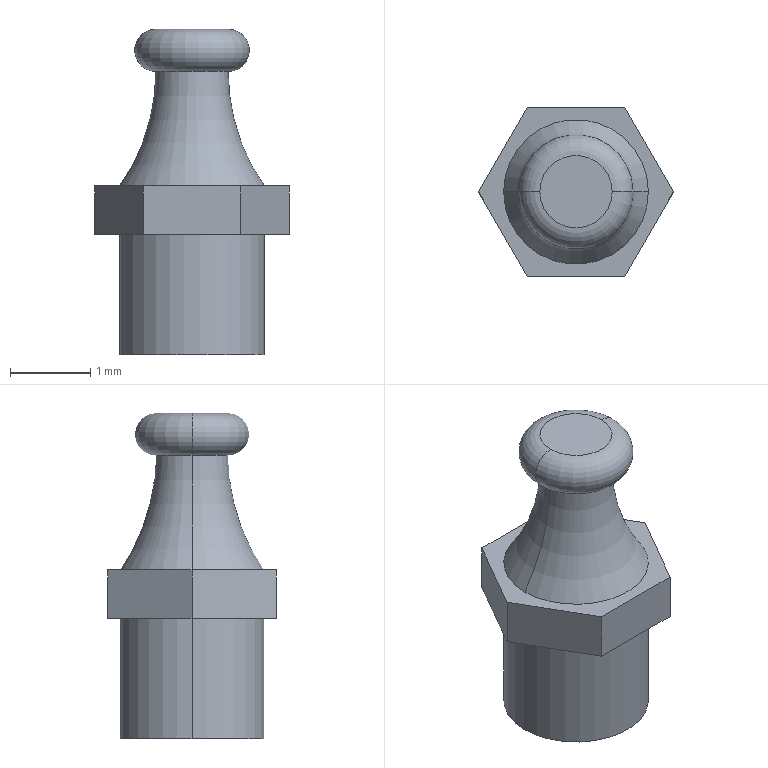Part | STEP file | 2026.6.15-Main Assembly图.sldasm-Part-210 | 1 solid | 16 faces | box 2.425 x 2.1 x 4.05 mm | volume 8.483 mm3 | plane 10 | torus 4 | cylinder 2 | commonest cylinder face diameters 1.8 x2
STEP:
#1=CARTESIAN_POINT('',(-1628.838,1424.264,3418.133));
#2=VERTEX_POINT('',#1);
#3=CARTESIAN_POINT('',(-1629.738,1424.264,3418.133));
#4=VERTEX_POINT('',#3);
#5=CARTESIAN_POINT('',(-1629.288,1424.264,3418.133));
#6=DIRECTION('',(0.,0.,-1.));
#7=DIRECTION('',(1.,0.,0.));
#8=AXIS2_PLACEMENT_3D('',#5,#6,#7);
#9=CIRCLE('',#8,0.45);
#10=EDGE_CURVE('',#2,#4,#9,.T.);
#11=ORIENTED_EDGE('',*,*,#10,.F.);
#12=CARTESIAN_POINT('',(-1629.288,1424.264,3418.133));
#13=DIRECTION('',(0.,0.,-1.));
#14=DIRECTION('',(1.,0.,0.));
#15=AXIS2_PLACEMENT_3D('',#12,#13,#14);
#16=CIRCLE('',#15,0.45);
#17=EDGE_CURVE('',#4,#2,#16,.T.);
#18=ORIENTED_EDGE('',*,*,#17,.F.);
#19=EDGE_LOOP('',(#11,#18));
#20=FACE_OUTER_BOUND('',#19,.T.);
#21=CARTESIAN_POINT('',(-1629.288,1424.264,3418.133));
#22=DIRECTION('',(0.,0.,-1.));
#23=DIRECTION('',(1.,0.,0.));
#24=AXIS2_PLACEMENT_3D('',#21,#22,#23);
#25=PLANE('',#24);
#26=ADVANCED_FACE('',(#20),#25,.F.);
#27=CARTESIAN_POINT('',(-1629.738,1424.264,3417.608));
#28=VERTEX_POINT('',#27);
#29=CARTESIAN_POINT('',(-1629.738,1424.264,3417.871));
#30=DIRECTION('',(0.,1.,0.));
#31=DIRECTION('',(0.9969,0.,-0.0785));
#32=AXIS2_PLACEMENT_3D('',#29,#30,#31);
#33=CIRCLE('',#32,0.2625);
#34=EDGE_CURVE('',#28,#4,#33,.T.);
#35=ORIENTED_EDGE('',*,*,#34,.F.);
#36=CARTESIAN_POINT('',(-1628.838,1424.264,3417.608));
#37=VERTEX_POINT('',#36);
#38=CARTESIAN_POINT('',(-1629.288,1424.264,3417.608));
#39=DIRECTION('',(0.,0.,1.));
#40=DIRECTION('',(1.,0.,0.));
#41=AXIS2_PLACEMENT_3D('',#38,#39,#40);
#42=CIRCLE('',#41,0.45);
#43=EDGE_CURVE('',#28,#37,#42,.T.);
#44=ORIENTED_EDGE('',*,*,#43,.T.);
#45=CARTESIAN_POINT('',(-1628.838,1424.264,3417.871));
#46=DIRECTION('',(0.,-1.,0.));
#47=DIRECTION('',(-0.9969,0.,0.0785));
#48=AXIS2_PLACEMENT_3D('',#45,#46,#47);
#49=CIRCLE('',#48,0.2625);
#50=EDGE_CURVE('',#37,#2,#49,.T.);
#51=ORIENTED_EDGE('',*,*,#50,.T.);
#52=ORIENTED_EDGE('',*,*,#10,.T.);
#53=EDGE_LOOP('',(#35,#44,#51,#52));
#54=FACE_OUTER_BOUND('',#53,.T.);
#55=CARTESIAN_POINT('',(-1629.288,1424.264,3417.871));
#56=DIRECTION('',(0.,0.,1.));
#57=DIRECTION('',(-1.,0.,0.));
#58=AXIS2_PLACEMENT_3D('',#55,#56,#57);
#59=TOROIDAL_SURFACE('',#58,0.45,0.2625);
#60=ADVANCED_FACE('',(#54),#59,.T.);
#61=CARTESIAN_POINT('',(-1630.188,1424.264,3416.183));
#62=VERTEX_POINT('',#61);
#63=CARTESIAN_POINT('',(-1632.22,1424.264,3417.608));
#64=DIRECTION('',(0.,1.,0.));
#65=DIRECTION('',(-0.0785,0.,-0.9969));
#66=AXIS2_PLACEMENT_3D('',#63,#64,#65);
#67=CIRCLE('',#66,2.481);
#68=EDGE_CURVE('',#28,#62,#67,.T.);
#69=ORIENTED_EDGE('',*,*,#68,.F.);
#70=CARTESIAN_POINT('',(-1629.288,1424.264,3417.608));
#71=DIRECTION('',(0.,0.,1.));
#72=DIRECTION('',(1.,0.,0.));
#73=AXIS2_PLACEMENT_3D('',#70,#71,#72);
#74=CIRCLE('',#73,0.45);
#75=EDGE_CURVE('',#37,#28,#74,.T.);
#76=ORIENTED_EDGE('',*,*,#75,.F.);
#77=CARTESIAN_POINT('',(-1628.388,1424.264,3416.183));
#78=VERTEX_POINT('',#77);
#79=CARTESIAN_POINT('',(-1626.357,1424.264,3417.608));
#80=DIRECTION('',(0.,-1.,0.));
#81=DIRECTION('',(0.0785,0.,0.9969));
#82=AXIS2_PLACEMENT_3D('',#79,#80,#81);
#83=CIRCLE('',#82,2.481);
#84=EDGE_CURVE('',#37,#78,#83,.T.);
#85=ORIENTED_EDGE('',*,*,#84,.T.);
#86=CARTESIAN_POINT('',(-1629.288,1424.264,3416.183));
#87=DIRECTION('',(0.,0.,1.));
#88=DIRECTION('',(1.,0.,0.));
#89=AXIS2_PLACEMENT_3D('',#86,#87,#88);
#90=CIRCLE('',#89,0.9);
#91=EDGE_CURVE('',#78,#62,#90,.T.);
#92=ORIENTED_EDGE('',*,*,#91,.T.);
#93=EDGE_LOOP('',(#69,#76,#85,#92));
#94=FACE_OUTER_BOUND('',#93,.T.);
#95=CARTESIAN_POINT('',(-1629.288,1424.264,3417.608));
#96=DIRECTION('',(0.,0.,1.));
#97=DIRECTION('',(-1.,0.,0.));
#98=AXIS2_PLACEMENT_3D('',#95,#96,#97);
#99=TOROIDAL_SURFACE('',#98,2.931,2.481);
#100=ADVANCED_FACE('',(#94),#99,.F.);
#101=CARTESIAN_POINT('',(-1630.501,1424.264,3416.183));
#102=VERTEX_POINT('',#101);
#103=CARTESIAN_POINT('',(-1629.894,1423.214,3416.183));
#104=VERTEX_POINT('',#103);
#105=CARTESIAN_POINT('',(-1630.501,1424.264,3416.183));
#106=DIRECTION('',(0.5,-0.866,0.));
#107=VECTOR('',#106,1000.);
#108=LINE('',#105,#107);
#109=EDGE_CURVE('',#102,#104,#108,.T.);
#110=ORIENTED_EDGE('',*,*,#109,.T.);
#111=CARTESIAN_POINT('',(-1628.682,1423.214,3416.183));
#112=VERTEX_POINT('',#111);
#113=CARTESIAN_POINT('',(-1629.894,1423.214,3416.183));
#114=DIRECTION('',(1.,0.,0.));
#115=VECTOR('',#114,1000.);
#116=LINE('',#113,#115);
#117=EDGE_CURVE('',#104,#112,#116,.T.);
#118=ORIENTED_EDGE('',*,*,#117,.T.);
#119=CARTESIAN_POINT('',(-1628.076,1424.264,3416.183));
#120=VERTEX_POINT('',#119);
#121=CARTESIAN_POINT('',(-1628.682,1423.214,3416.183));
#122=DIRECTION('',(0.5,0.866,0.));
#123=VECTOR('',#122,1000.);
#124=LINE('',#121,#123);
#125=EDGE_CURVE('',#112,#120,#124,.T.);
#126=ORIENTED_EDGE('',*,*,#125,.T.);
#127=CARTESIAN_POINT('',(-1628.682,1425.314,3416.183));
#128=VERTEX_POINT('',#127);
#129=CARTESIAN_POINT('',(-1628.076,1424.264,3416.183));
#130=DIRECTION('',(-0.5,0.866,0.));
#131=VECTOR('',#130,1000.);
#132=LINE('',#129,#131);
#133=EDGE_CURVE('',#120,#128,#132,.T.);
#134=ORIENTED_EDGE('',*,*,#133,.T.);
#135=CARTESIAN_POINT('',(-1629.894,1425.314,3416.183));
#136=VERTEX_POINT('',#135);
#137=CARTESIAN_POINT('',(-1628.682,1425.314,3416.183));
#138=DIRECTION('',(-1.,0.,0.));
#139=VECTOR('',#138,1000.);
#140=LINE('',#137,#139);
#141=EDGE_CURVE('',#128,#136,#140,.T.);
#142=ORIENTED_EDGE('',*,*,#141,.T.);
#143=CARTESIAN_POINT('',(-1629.894,1425.314,3416.183));
#144=DIRECTION('',(-0.5,-0.866,0.));
#145=VECTOR('',#144,1000.);
#146=LINE('',#143,#145);
#147=EDGE_CURVE('',#136,#102,#146,.T.);
#148=ORIENTED_EDGE('',*,*,#147,.T.);
#149=EDGE_LOOP('',(#110,#118,#126,#134,#142,#148));
#150=FACE_OUTER_BOUND('',#149,.T.);
#151=ORIENTED_EDGE('',*,*,#91,.F.);
#152=CARTESIAN_POINT('',(-1629.288,1424.264,3416.183));
#153=DIRECTION('',(0.,0.,1.));
#154=DIRECTION('',(1.,0.,0.));
#155=AXIS2_PLACEMENT_3D('',#152,#153,#154);
#156=CIRCLE('',#155,0.9);
#157=EDGE_CURVE('',#62,#78,#156,.T.);
#158=ORIENTED_EDGE('',*,*,#157,.F.);
#159=EDGE_LOOP('',(#151,#158));
#160=FACE_BOUND('',#159,.T.);
#161=CARTESIAN_POINT('',(-1628.682,1425.314,3416.183));
#162=DIRECTION('',(0.,0.,-1.));
#163=DIRECTION('',(1.,0.,0.));
#164=AXIS2_PLACEMENT_3D('',#161,#162,#163);
#165=PLANE('',#164);
#166=ADVANCED_FACE('',(#150,#160),#165,.F.);
#167=CARTESIAN_POINT('',(-1629.894,1423.214,3415.583));
#168=VERTEX_POINT('',#167);
#169=CARTESIAN_POINT('',(-1629.894,1423.214,3415.583));
#170=DIRECTION('',(0.,0.,1.));
#171=VECTOR('',#170,1000.);
#172=LINE('',#169,#171);
#173=EDGE_CURVE('',#168,#104,#172,.T.);
#174=ORIENTED_EDGE('',*,*,#173,.T.);
#175=ORIENTED_EDGE('',*,*,#109,.F.);
#176=CARTESIAN_POINT('',(-1630.501,1424.264,3415.583));
#177=VERTEX_POINT('',#176);
#178=CARTESIAN_POINT('',(-1630.501,1424.264,3416.183));
#179=DIRECTION('',(0.,0.,-1.));
#180=VECTOR('',#179,1000.);
#181=LINE('',#178,#180);
#182=EDGE_CURVE('',#102,#177,#181,.T.);
#183=ORIENTED_EDGE('',*,*,#182,.T.);
#184=CARTESIAN_POINT('',(-1629.894,1423.214,3415.583));
#185=DIRECTION('',(-0.5,0.866,0.));
#186=VECTOR('',#185,1000.);
#187=LINE('',#184,#186);
#188=EDGE_CURVE('',#168,#177,#187,.T.);
#189=ORIENTED_EDGE('',*,*,#188,.F.);
#190=EDGE_LOOP('',(#174,#175,#183,#189));
#191=FACE_OUTER_BOUND('',#190,.T.);
#192=CARTESIAN_POINT('',(-1629.894,1423.214,3415.583));
#193=DIRECTION('',(0.866,0.5,0.));
#194=DIRECTION('',(0.,0.,1.));
#195=AXIS2_PLACEMENT_3D('',#192,#193,#194);
#196=PLANE('',#195);
#197=ADVANCED_FACE('',(#191),#196,.F.);
#198=ORIENTED_EDGE('',*,*,#147,.F.);
#199=CARTESIAN_POINT('',(-1629.894,1425.314,3415.583));
#200=VERTEX_POINT('',#199);
#201=CARTESIAN_POINT('',(-1629.894,1425.314,3416.183));
#202=DIRECTION('',(0.,0.,-1.));
#203=VECTOR('',#202,1000.);
#204=LINE('',#201,#203);
#205=EDGE_CURVE('',#136,#200,#204,.T.);
#206=ORIENTED_EDGE('',*,*,#205,.T.);
#207=CARTESIAN_POINT('',(-1630.501,1424.264,3415.583));
#208=DIRECTION('',(0.5,0.866,0.));
#209=VECTOR('',#208,1000.);
#210=LINE('',#207,#209);
#211=EDGE_CURVE('',#177,#200,#210,.T.);
#212=ORIENTED_EDGE('',*,*,#211,.F.);
#213=ORIENTED_EDGE('',*,*,#182,.F.);
#214=EDGE_LOOP('',(#198,#206,#212,#213));
#215=FACE_OUTER_BOUND('',#214,.T.);
#216=CARTESIAN_POINT('',(-1630.501,1424.264,3415.583));
#217=DIRECTION('',(0.866,-0.5,0.));
#218=DIRECTION('',(-0.5,-0.866,0.));
#219=AXIS2_PLACEMENT_3D('',#216,#217,#218);
#220=PLANE('',#219);
#221=ADVANCED_FACE('',(#215),#220,.F.);
#222=ORIENTED_EDGE('',*,*,#205,.F.);
#223=ORIENTED_EDGE('',*,*,#141,.F.);
#224=CARTESIAN_POINT('',(-1628.682,1425.314,3415.583));
#225=VERTEX_POINT('',#224);
#226=CARTESIAN_POINT('',(-1628.682,1425.314,3416.183));
#227=DIRECTION('',(0.,0.,-1.));
#228=VECTOR('',#227,1000.);
#229=LINE('',#226,#228);
#230=EDGE_CURVE('',#128,#225,#229,.T.);
#231=ORIENTED_EDGE('',*,*,#230,.T.);
#232=CARTESIAN_POINT('',(-1628.682,1425.314,3415.583));
#233=DIRECTION('',(1.,0.,0.));
#234=VECTOR('',#233,1000.);
#235=LINE('',#232,#234);
#236=EDGE_CURVE('',#200,#225,#235,.T.);
#237=ORIENTED_EDGE('',*,*,#236,.F.);
#238=EDGE_LOOP('',(#222,#223,#231,#237));
#239=FACE_OUTER_BOUND('',#238,.T.);
#240=CARTESIAN_POINT('',(-1629.894,1425.314,3415.583));
#241=DIRECTION('',(0.,-1.,0.));
#242=DIRECTION('',(-1.,0.,0.));
#243=AXIS2_PLACEMENT_3D('',#240,#241,#242);
#244=PLANE('',#243);
#245=ADVANCED_FACE('',(#239),#244,.F.);
#246=ORIENTED_EDGE('',*,*,#230,.F.);
#247=ORIENTED_EDGE('',*,*,#133,.F.);
#248=CARTESIAN_POINT('',(-1628.076,1424.264,3415.583));
#249=VERTEX_POINT('',#248);
#250=CARTESIAN_POINT('',(-1628.076,1424.264,3416.183));
#251=DIRECTION('',(0.,0.,-1.));
#252=VECTOR('',#251,1000.);
#253=LINE('',#250,#252);
#254=EDGE_CURVE('',#120,#249,#253,.T.);
#255=ORIENTED_EDGE('',*,*,#254,.T.);
#256=CARTESIAN_POINT('',(-1628.682,1425.314,3415.583));
#257=DIRECTION('',(0.5,-0.866,0.));
#258=VECTOR('',#257,1000.);
#259=LINE('',#256,#258);
#260=EDGE_CURVE('',#225,#249,#259,.T.);
#261=ORIENTED_EDGE('',*,*,#260,.F.);
#262=EDGE_LOOP('',(#246,#247,#255,#261));
#263=FACE_OUTER_BOUND('',#262,.T.);
#264=CARTESIAN_POINT('',(-1628.682,1425.314,3415.583));
#265=DIRECTION('',(-0.866,-0.5,0.));
#266=DIRECTION('',(0.,0.,-1.));
#267=AXIS2_PLACEMENT_3D('',#264,#265,#266);
#268=PLANE('',#267);
#269=ADVANCED_FACE('',(#263),#268,.F.);
#270=ORIENTED_EDGE('',*,*,#254,.F.);
#271=ORIENTED_EDGE('',*,*,#125,.F.);
#272=CARTESIAN_POINT('',(-1628.682,1423.214,3415.583));
#273=VERTEX_POINT('',#272);
#274=CARTESIAN_POINT('',(-1628.682,1423.214,3416.183));
#275=DIRECTION('',(0.,0.,-1.));
#276=VECTOR('',#275,1000.);
#277=LINE('',#274,#276);
#278=EDGE_CURVE('',#112,#273,#277,.T.);
#279=ORIENTED_EDGE('',*,*,#278,.T.);
#280=CARTESIAN_POINT('',(-1628.076,1424.264,3415.583));
#281=DIRECTION('',(-0.5,-0.866,0.));
#282=VECTOR('',#281,1000.);
#283=LINE('',#280,#282);
#284=EDGE_CURVE('',#249,#273,#283,.T.);
#285=ORIENTED_EDGE('',*,*,#284,.F.);
#286=EDGE_LOOP('',(#270,#271,#279,#285));
#287=FACE_OUTER_BOUND('',#286,.T.);
#288=CARTESIAN_POINT('',(-1628.076,1424.264,3415.583));
#289=DIRECTION('',(-0.866,0.5,0.));
#290=DIRECTION('',(0.,0.,-1.));
#291=AXIS2_PLACEMENT_3D('',#288,#289,#290);
#292=PLANE('',#291);
#293=ADVANCED_FACE('',(#287),#292,.F.);
#294=ORIENTED_EDGE('',*,*,#278,.F.);
#295=ORIENTED_EDGE('',*,*,#117,.F.);
#296=ORIENTED_EDGE('',*,*,#173,.F.);
#297=CARTESIAN_POINT('',(-1628.682,1423.214,3415.583));
#298=DIRECTION('',(-1.,0.,0.));
#299=VECTOR('',#298,1000.);
#300=LINE('',#297,#299);
#301=EDGE_CURVE('',#273,#168,#300,.T.);
#302=ORIENTED_EDGE('',*,*,#301,.F.);
#303=EDGE_LOOP('',(#294,#295,#296,#302));
#304=FACE_OUTER_BOUND('',#303,.T.);
#305=CARTESIAN_POINT('',(-1628.682,1423.214,3415.583));
#306=DIRECTION('',(0.,1.,0.));
#307=DIRECTION('',(1.,0.,0.));
#308=AXIS2_PLACEMENT_3D('',#305,#306,#307);
#309=PLANE('',#308);
#310=ADVANCED_FACE('',(#304),#309,.F.);
#311=ORIENTED_EDGE('',*,*,#284,.T.);
#312=ORIENTED_EDGE('',*,*,#301,.T.);
#313=ORIENTED_EDGE('',*,*,#188,.T.);
#314=ORIENTED_EDGE('',*,*,#211,.T.);
#315=ORIENTED_EDGE('',*,*,#236,.T.);
#316=ORIENTED_EDGE('',*,*,#260,.T.);
#317=EDGE_LOOP('',(#311,#312,#313,#314,#315,#316));
#318=FACE_OUTER_BOUND('',#317,.T.);
#319=CARTESIAN_POINT('',(-1630.188,1424.264,3415.583));
#320=VERTEX_POINT('',#319);
#321=CARTESIAN_POINT('',(-1628.388,1424.264,3415.583));
#322=VERTEX_POINT('',#321);
#323=CARTESIAN_POINT('',(-1629.288,1424.264,3415.583));
#324=DIRECTION('',(0.,0.,-1.));
#325=DIRECTION('',(-1.,0.,0.));
#326=AXIS2_PLACEMENT_3D('',#323,#324,#325);
#327=CIRCLE('',#326,0.9);
#328=EDGE_CURVE('',#320,#322,#327,.T.);
#329=ORIENTED_EDGE('',*,*,#328,.F.);
#330=CARTESIAN_POINT('',(-1629.288,1424.264,3415.583));
#331=DIRECTION('',(0.,0.,-1.));
#332=DIRECTION('',(-1.,0.,0.));
#333=AXIS2_PLACEMENT_3D('',#330,#331,#332);
#334=CIRCLE('',#333,0.9);
#335=EDGE_CURVE('',#322,#320,#334,.T.);
#336=ORIENTED_EDGE('',*,*,#335,.F.);
#337=EDGE_LOOP('',(#329,#336));
#338=FACE_BOUND('',#337,.T.);
#339=CARTESIAN_POINT('',(-1628.682,1425.314,3415.583));
#340=DIRECTION('',(0.,0.,-1.));
#341=DIRECTION('',(1.,0.,0.));
#342=AXIS2_PLACEMENT_3D('',#339,#340,#341);
#343=PLANE('',#342);
#344=ADVANCED_FACE('',(#318,#338),#343,.T.);
#345=CARTESIAN_POINT('',(-1630.188,1424.264,3414.083));
#346=VERTEX_POINT('',#345);
#347=CARTESIAN_POINT('',(-1628.388,1424.264,3414.083));
#348=VERTEX_POINT('',#347);
#349=CARTESIAN_POINT('',(-1629.288,1424.264,3414.083));
#350=DIRECTION('',(0.,0.,1.));
#351=DIRECTION('',(-1.,0.,0.));
#352=AXIS2_PLACEMENT_3D('',#349,#350,#351);
#353=CIRCLE('',#352,0.9);
#354=EDGE_CURVE('',#346,#348,#353,.T.);
#355=ORIENTED_EDGE('',*,*,#354,.F.);
#356=CARTESIAN_POINT('',(-1629.288,1424.264,3414.083));
#357=DIRECTION('',(0.,0.,1.));
#358=DIRECTION('',(-1.,0.,0.));
#359=AXIS2_PLACEMENT_3D('',#356,#357,#358);
#360=CIRCLE('',#359,0.9);
#361=EDGE_CURVE('',#348,#346,#360,.T.);
#362=ORIENTED_EDGE('',*,*,#361,.F.);
#363=EDGE_LOOP('',(#355,#362));
#364=FACE_OUTER_BOUND('',#363,.T.);
#365=CARTESIAN_POINT('',(-1630.188,1424.264,3414.083));
#366=DIRECTION('',(0.,0.,1.));
#367=DIRECTION('',(0.,1.,0.));
#368=AXIS2_PLACEMENT_3D('',#365,#366,#367);
#369=PLANE('',#368);
#370=ADVANCED_FACE('',(#364),#369,.F.);
#371=CARTESIAN_POINT('',(-1628.388,1424.264,3435.233));
#372=DIRECTION('',(0.,0.,1.));
#373=VECTOR('',#372,1000.);
#374=LINE('',#371,#373);
#375=EDGE_CURVE('',#348,#322,#374,.T.);
#376=ORIENTED_EDGE('',*,*,#375,.T.);
#377=ORIENTED_EDGE('',*,*,#335,.T.);
#378=CARTESIAN_POINT('',(-1630.188,1424.264,3435.233));
#379=DIRECTION('',(0.,0.,1.));
#380=VECTOR('',#379,1000.);
#381=LINE('',#378,#380);
#382=EDGE_CURVE('',#346,#320,#381,.T.);
#383=ORIENTED_EDGE('',*,*,#382,.F.);
#384=ORIENTED_EDGE('',*,*,#354,.T.);
#385=EDGE_LOOP('',(#376,#377,#383,#384));
#386=FACE_OUTER_BOUND('',#385,.T.);
#387=CARTESIAN_POINT('',(-1629.288,1424.264,3435.233));
#388=DIRECTION('',(0.,0.,-1.));
#389=DIRECTION('',(1.,0.,0.));
#390=AXIS2_PLACEMENT_3D('',#387,#388,#389);
#391=CYLINDRICAL_SURFACE('',#390,0.9);
#392=ADVANCED_FACE('',(#386),#391,.T.);
#393=ORIENTED_EDGE('',*,*,#75,.T.);
#394=ORIENTED_EDGE('',*,*,#34,.T.);
#395=ORIENTED_EDGE('',*,*,#17,.T.);
#396=ORIENTED_EDGE('',*,*,#50,.F.);
#397=EDGE_LOOP('',(#393,#394,#395,#396));
#398=FACE_OUTER_BOUND('',#397,.T.);
#399=CARTESIAN_POINT('',(-1629.288,1424.264,3417.871));
#400=DIRECTION('',(0.,0.,1.));
#401=DIRECTION('',(-1.,0.,0.));
#402=AXIS2_PLACEMENT_3D('',#399,#400,#401);
#403=TOROIDAL_SURFACE('',#402,0.45,0.2625);
#404=ADVANCED_FACE('',(#398),#403,.T.);
#405=ORIENTED_EDGE('',*,*,#43,.F.);
#406=ORIENTED_EDGE('',*,*,#68,.T.);
#407=ORIENTED_EDGE('',*,*,#157,.T.);
#408=ORIENTED_EDGE('',*,*,#84,.F.);
#409=EDGE_LOOP('',(#405,#406,#407,#408));
#410=FACE_OUTER_BOUND('',#409,.T.);
#411=CARTESIAN_POINT('',(-1629.288,1424.264,3417.608));
#412=DIRECTION('',(0.,0.,1.));
#413=DIRECTION('',(-1.,0.,0.));
#414=AXIS2_PLACEMENT_3D('',#411,#412,#413);
#415=TOROIDAL_SURFACE('',#414,2.931,2.481);
#416=ADVANCED_FACE('',(#410),#415,.F.);
#417=ORIENTED_EDGE('',*,*,#328,.T.);
#418=ORIENTED_EDGE('',*,*,#375,.F.);
#419=ORIENTED_EDGE('',*,*,#361,.T.);
#420=ORIENTED_EDGE('',*,*,#382,.T.);
#421=EDGE_LOOP('',(#417,#418,#419,#420));
#422=FACE_OUTER_BOUND('',#421,.T.);
#423=CARTESIAN_POINT('',(-1629.288,1424.264,3435.233));
#424=DIRECTION('',(0.,0.,-1.));
#425=DIRECTION('',(1.,0.,0.));
#426=AXIS2_PLACEMENT_3D('',#423,#424,#425);
#427=CYLINDRICAL_SURFACE('',#426,0.9);
#428=ADVANCED_FACE('',(#422),#427,.T.);
#429=CLOSED_SHELL('',(#26,#60,#100,#166,#197,#221,#245,#269,#293,#310,#344,#370,#392,#404,#416,#428));
#430=MANIFOLD_SOLID_BREP('',#429);
#431=CARTESIAN_POINT('',(0.,0.,0.));
#432=DIRECTION('',(0.,0.,1.));
#433=DIRECTION('',(1.,0.,0.));
#434=AXIS2_PLACEMENT_3D('',#431,#432,#433);
#435=(LENGTH_UNIT()NAMED_UNIT(*)SI_UNIT(.MILLI.,.METRE.));
#436=UNCERTAINTY_MEASURE_WITH_UNIT(LENGTH_MEASURE(0.00001),#435,'','');
#437=(NAMED_UNIT(*)PLANE_ANGLE_UNIT()SI_UNIT($,.RADIAN.));
#438=(NAMED_UNIT(*)SI_UNIT($,.STERADIAN.)SOLID_ANGLE_UNIT());
#439=(GEOMETRIC_REPRESENTATION_CONTEXT(3)GLOBAL_UNCERTAINTY_ASSIGNED_CONTEXT((#436))GLOBAL_UNIT_ASSIGNED_CONTEXT((#435,#437,#438))REPRESENTATION_CONTEXT('',''));
#440=ADVANCED_BREP_SHAPE_REPRESENTATION('',(#430,#434),#439);